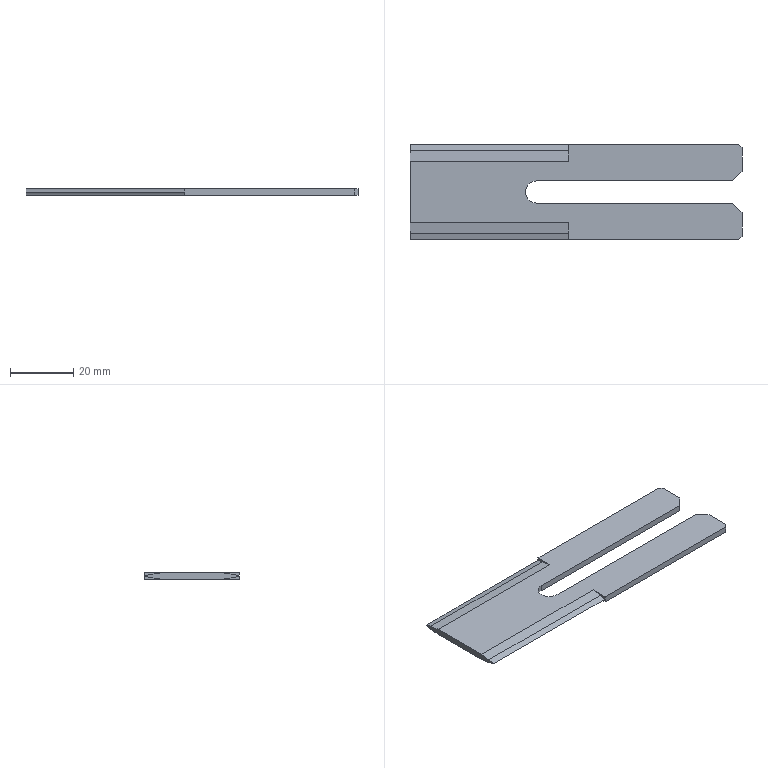Part | SolidWorks | features Chamfer 2, ICE 2, Extrusion 1 | 1 solid | 27 faces | box 105 x 30 x 2 mm | volume 4885 mm3 | plane 25 | cylinder 2 | commonest cylinder face diameters 7 x2
STEP:
#1=CARTESIAN_POINT('',(-16.,0.,2.));
#2=VERTEX_POINT('',#1);
#3=CARTESIAN_POINT('',(-12.5,3.5,2.));
#4=VERTEX_POINT('',#3);
#5=CARTESIAN_POINT('',(-12.5,0.,2.));
#6=DIRECTION('',(0.,0.,-1.));
#7=DIRECTION('',(1.,0.,0.));
#8=AXIS2_PLACEMENT_3D('',#5,#6,#7);
#9=CIRCLE('',#8,3.5);
#10=EDGE_CURVE('',#2,#4,#9,.T.);
#11=ORIENTED_EDGE('',*,*,#10,.F.);
#12=CARTESIAN_POINT('',(-16.,0.,0.));
#13=VERTEX_POINT('',#12);
#14=CARTESIAN_POINT('',(-16.,0.,141.025));
#15=DIRECTION('',(0.,0.,-1.));
#16=VECTOR('',#15,1000.);
#17=LINE('',#14,#16);
#18=EDGE_CURVE('',#2,#13,#17,.T.);
#19=ORIENTED_EDGE('',*,*,#18,.T.);
#20=CARTESIAN_POINT('',(-12.5,3.5,0.));
#21=VERTEX_POINT('',#20);
#22=CARTESIAN_POINT('',(-12.5,0.,0.));
#23=DIRECTION('',(0.,0.,-1.));
#24=DIRECTION('',(1.,0.,0.));
#25=AXIS2_PLACEMENT_3D('',#22,#23,#24);
#26=CIRCLE('',#25,3.5);
#27=EDGE_CURVE('',#13,#21,#26,.T.);
#28=ORIENTED_EDGE('',*,*,#27,.T.);
#29=CARTESIAN_POINT('',(-12.5,3.5,141.025));
#30=DIRECTION('',(0.,0.,-1.));
#31=VECTOR('',#30,1000.);
#32=LINE('',#29,#31);
#33=EDGE_CURVE('',#4,#21,#32,.T.);
#34=ORIENTED_EDGE('',*,*,#33,.F.);
#35=EDGE_LOOP('',(#11,#19,#28,#34));
#36=FACE_OUTER_BOUND('',#35,.T.);
#37=CARTESIAN_POINT('',(-12.5,0.,141.025));
#38=DIRECTION('',(0.,0.,-1.));
#39=DIRECTION('',(-1.,0.,0.));
#40=AXIS2_PLACEMENT_3D('',#37,#38,#39);
#41=CYLINDRICAL_SURFACE('',#40,3.5);
#42=ADVANCED_FACE('',(#36),#41,.F.);
#43=CARTESIAN_POINT('',(49.5,3.5,2.));
#44=VERTEX_POINT('',#43);
#45=CARTESIAN_POINT('',(0.,3.5,2.));
#46=DIRECTION('',(1.,0.,0.));
#47=VECTOR('',#46,1000.);
#48=LINE('',#45,#47);
#49=EDGE_CURVE('',#4,#44,#48,.T.);
#50=ORIENTED_EDGE('',*,*,#49,.T.);
#51=CARTESIAN_POINT('',(52.5,6.5,2.));
#52=VERTEX_POINT('',#51);
#53=CARTESIAN_POINT('',(23.,-23.,2.));
#54=DIRECTION('',(0.7071,0.7071,0.));
#55=VECTOR('',#54,1000.);
#56=LINE('',#53,#55);
#57=EDGE_CURVE('',#44,#52,#56,.T.);
#58=ORIENTED_EDGE('',*,*,#57,.T.);
#59=CARTESIAN_POINT('',(52.5,14.,2.));
#60=VERTEX_POINT('',#59);
#61=CARTESIAN_POINT('',(52.5,15.,2.));
#62=DIRECTION('',(0.,1.,0.));
#63=VECTOR('',#62,1000.);
#64=LINE('',#61,#63);
#65=EDGE_CURVE('',#52,#60,#64,.T.);
#66=ORIENTED_EDGE('',*,*,#65,.T.);
#67=CARTESIAN_POINT('',(51.5,15.,2.));
#68=VERTEX_POINT('',#67);
#69=CARTESIAN_POINT('',(33.25,33.25,2.));
#70=DIRECTION('',(-0.7071,0.7071,0.));
#71=VECTOR('',#70,1000.);
#72=LINE('',#69,#71);
#73=EDGE_CURVE('',#60,#68,#72,.T.);
#74=ORIENTED_EDGE('',*,*,#73,.T.);
#75=CARTESIAN_POINT('',(-2.5,15.,2.));
#76=VERTEX_POINT('',#75);
#77=CARTESIAN_POINT('',(-52.5,15.,2.));
#78=DIRECTION('',(-1.,0.,0.));
#79=VECTOR('',#78,1000.);
#80=LINE('',#77,#79);
#81=EDGE_CURVE('',#68,#76,#80,.T.);
#82=ORIENTED_EDGE('',*,*,#81,.T.);
#83=CARTESIAN_POINT('',(-2.5,9.698,2.));
#84=VERTEX_POINT('',#83);
#85=CARTESIAN_POINT('',(-2.5,0.,2.));
#86=DIRECTION('',(0.,-1.,0.));
#87=VECTOR('',#86,1000.);
#88=LINE('',#85,#87);
#89=EDGE_CURVE('',#76,#84,#88,.T.);
#90=ORIENTED_EDGE('',*,*,#89,.T.);
#91=CARTESIAN_POINT('',(-52.5,9.698,2.));
#92=VERTEX_POINT('',#91);
#93=CARTESIAN_POINT('',(-2.5,9.698,2.));
#94=DIRECTION('',(-1.,0.,0.));
#95=VECTOR('',#94,1000.);
#96=LINE('',#93,#95);
#97=EDGE_CURVE('',#84,#92,#96,.T.);
#98=ORIENTED_EDGE('',*,*,#97,.T.);
#99=CARTESIAN_POINT('',(-52.5,-9.698,2.));
#100=VERTEX_POINT('',#99);
#101=CARTESIAN_POINT('',(-52.5,15.,2.));
#102=DIRECTION('',(0.,-1.,0.));
#103=VECTOR('',#102,1000.);
#104=LINE('',#101,#103);
#105=EDGE_CURVE('',#92,#100,#104,.T.);
#106=ORIENTED_EDGE('',*,*,#105,.T.);
#107=CARTESIAN_POINT('',(-2.5,-9.698,2.));
#108=VERTEX_POINT('',#107);
#109=CARTESIAN_POINT('',(-2.5,-9.698,2.));
#110=DIRECTION('',(-1.,0.,0.));
#111=VECTOR('',#110,1000.);
#112=LINE('',#109,#111);
#113=EDGE_CURVE('',#108,#100,#112,.T.);
#114=ORIENTED_EDGE('',*,*,#113,.F.);
#115=CARTESIAN_POINT('',(-2.5,-15.,2.));
#116=VERTEX_POINT('',#115);
#117=CARTESIAN_POINT('',(-2.5,0.,2.));
#118=DIRECTION('',(0.,-1.,0.));
#119=VECTOR('',#118,1000.);
#120=LINE('',#117,#119);
#121=EDGE_CURVE('',#108,#116,#120,.T.);
#122=ORIENTED_EDGE('',*,*,#121,.T.);
#123=CARTESIAN_POINT('',(51.5,-15.,2.));
#124=VERTEX_POINT('',#123);
#125=CARTESIAN_POINT('',(-52.5,-15.,2.));
#126=DIRECTION('',(1.,0.,0.));
#127=VECTOR('',#126,1000.);
#128=LINE('',#125,#127);
#129=EDGE_CURVE('',#116,#124,#128,.T.);
#130=ORIENTED_EDGE('',*,*,#129,.T.);
#131=CARTESIAN_POINT('',(52.5,-14.,2.));
#132=VERTEX_POINT('',#131);
#133=CARTESIAN_POINT('',(33.25,-33.25,2.));
#134=DIRECTION('',(0.7071,0.7071,0.));
#135=VECTOR('',#134,1000.);
#136=LINE('',#133,#135);
#137=EDGE_CURVE('',#124,#132,#136,.T.);
#138=ORIENTED_EDGE('',*,*,#137,.T.);
#139=CARTESIAN_POINT('',(52.5,-6.5,2.));
#140=VERTEX_POINT('',#139);
#141=CARTESIAN_POINT('',(52.5,15.,2.));
#142=DIRECTION('',(0.,1.,0.));
#143=VECTOR('',#142,1000.);
#144=LINE('',#141,#143);
#145=EDGE_CURVE('',#132,#140,#144,.T.);
#146=ORIENTED_EDGE('',*,*,#145,.T.);
#147=CARTESIAN_POINT('',(49.5,-3.5,2.));
#148=VERTEX_POINT('',#147);
#149=CARTESIAN_POINT('',(23.,23.,2.));
#150=DIRECTION('',(-0.7071,0.7071,0.));
#151=VECTOR('',#150,1000.);
#152=LINE('',#149,#151);
#153=EDGE_CURVE('',#140,#148,#152,.T.);
#154=ORIENTED_EDGE('',*,*,#153,.T.);
#155=CARTESIAN_POINT('',(-12.5,-3.5,2.));
#156=VERTEX_POINT('',#155);
#157=CARTESIAN_POINT('',(0.,-3.5,2.));
#158=DIRECTION('',(-1.,0.,0.));
#159=VECTOR('',#158,1000.);
#160=LINE('',#157,#159);
#161=EDGE_CURVE('',#148,#156,#160,.T.);
#162=ORIENTED_EDGE('',*,*,#161,.T.);
#163=CARTESIAN_POINT('',(-12.5,0.,2.));
#164=DIRECTION('',(0.,0.,-1.));
#165=DIRECTION('',(1.,0.,0.));
#166=AXIS2_PLACEMENT_3D('',#163,#164,#165);
#167=CIRCLE('',#166,3.5);
#168=EDGE_CURVE('',#156,#2,#167,.T.);
#169=ORIENTED_EDGE('',*,*,#168,.T.);
#170=ORIENTED_EDGE('',*,*,#10,.T.);
#171=EDGE_LOOP('',(#50,#58,#66,#74,#82,#90,#98,#106,#114,#122,#130,#138,#146,#154,#162,#169,#170));
#172=FACE_OUTER_BOUND('',#171,.T.);
#173=CARTESIAN_POINT('',(0.,0.,2.));
#174=DIRECTION('',(0.,0.,1.));
#175=DIRECTION('',(1.,0.,0.));
#176=AXIS2_PLACEMENT_3D('',#173,#174,#175);
#177=PLANE('',#176);
#178=ADVANCED_FACE('',(#172),#177,.T.);
#179=CARTESIAN_POINT('',(52.5,6.5,0.));
#180=VERTEX_POINT('',#179);
#181=CARTESIAN_POINT('',(52.5,14.,0.));
#182=VERTEX_POINT('',#181);
#183=CARTESIAN_POINT('',(52.5,15.,0.));
#184=DIRECTION('',(0.,1.,0.));
#185=VECTOR('',#184,1000.);
#186=LINE('',#183,#185);
#187=EDGE_CURVE('',#180,#182,#186,.T.);
#188=ORIENTED_EDGE('',*,*,#187,.F.);
#189=CARTESIAN_POINT('',(49.5,3.5,0.));
#190=VERTEX_POINT('',#189);
#191=CARTESIAN_POINT('',(52.5,6.5,0.));
#192=DIRECTION('',(-0.7071,-0.7071,0.));
#193=VECTOR('',#192,1000.);
#194=LINE('',#191,#193);
#195=EDGE_CURVE('',#180,#190,#194,.T.);
#196=ORIENTED_EDGE('',*,*,#195,.T.);
#197=CARTESIAN_POINT('',(0.,3.5,0.));
#198=DIRECTION('',(1.,0.,0.));
#199=VECTOR('',#198,1000.);
#200=LINE('',#197,#199);
#201=EDGE_CURVE('',#21,#190,#200,.T.);
#202=ORIENTED_EDGE('',*,*,#201,.F.);
#203=ORIENTED_EDGE('',*,*,#27,.F.);
#204=CARTESIAN_POINT('',(-12.5,-3.5,0.));
#205=VERTEX_POINT('',#204);
#206=CARTESIAN_POINT('',(-12.5,0.,0.));
#207=DIRECTION('',(0.,0.,-1.));
#208=DIRECTION('',(1.,0.,0.));
#209=AXIS2_PLACEMENT_3D('',#206,#207,#208);
#210=CIRCLE('',#209,3.5);
#211=EDGE_CURVE('',#205,#13,#210,.T.);
#212=ORIENTED_EDGE('',*,*,#211,.F.);
#213=CARTESIAN_POINT('',(49.5,-3.5,0.));
#214=VERTEX_POINT('',#213);
#215=CARTESIAN_POINT('',(0.,-3.5,0.));
#216=DIRECTION('',(-1.,0.,0.));
#217=VECTOR('',#216,1000.);
#218=LINE('',#215,#217);
#219=EDGE_CURVE('',#214,#205,#218,.T.);
#220=ORIENTED_EDGE('',*,*,#219,.F.);
#221=CARTESIAN_POINT('',(52.5,-6.5,0.));
#222=VERTEX_POINT('',#221);
#223=CARTESIAN_POINT('',(49.5,-3.5,0.));
#224=DIRECTION('',(0.7071,-0.7071,0.));
#225=VECTOR('',#224,1000.);
#226=LINE('',#223,#225);
#227=EDGE_CURVE('',#214,#222,#226,.T.);
#228=ORIENTED_EDGE('',*,*,#227,.T.);
#229=CARTESIAN_POINT('',(52.5,-14.,0.));
#230=VERTEX_POINT('',#229);
#231=CARTESIAN_POINT('',(52.5,15.,0.));
#232=DIRECTION('',(0.,1.,0.));
#233=VECTOR('',#232,1000.);
#234=LINE('',#231,#233);
#235=EDGE_CURVE('',#230,#222,#234,.T.);
#236=ORIENTED_EDGE('',*,*,#235,.F.);
#237=CARTESIAN_POINT('',(51.5,-15.,0.));
#238=VERTEX_POINT('',#237);
#239=CARTESIAN_POINT('',(52.5,-14.,0.));
#240=DIRECTION('',(-0.7071,-0.7071,0.));
#241=VECTOR('',#240,1000.);
#242=LINE('',#239,#241);
#243=EDGE_CURVE('',#230,#238,#242,.T.);
#244=ORIENTED_EDGE('',*,*,#243,.T.);
#245=CARTESIAN_POINT('',(-2.5,-15.,0.));
#246=VERTEX_POINT('',#245);
#247=CARTESIAN_POINT('',(-52.5,-15.,0.));
#248=DIRECTION('',(1.,0.,0.));
#249=VECTOR('',#248,1000.);
#250=LINE('',#247,#249);
#251=EDGE_CURVE('',#246,#238,#250,.T.);
#252=ORIENTED_EDGE('',*,*,#251,.F.);
#253=CARTESIAN_POINT('',(-2.5,-9.698,0.));
#254=VERTEX_POINT('',#253);
#255=CARTESIAN_POINT('',(-2.5,0.,0.));
#256=DIRECTION('',(0.,-1.,0.));
#257=VECTOR('',#256,1000.);
#258=LINE('',#255,#257);
#259=EDGE_CURVE('',#254,#246,#258,.T.);
#260=ORIENTED_EDGE('',*,*,#259,.F.);
#261=CARTESIAN_POINT('',(-52.5,-9.698,0.));
#262=VERTEX_POINT('',#261);
#263=CARTESIAN_POINT('',(-2.5,-9.698,0.));
#264=DIRECTION('',(-1.,0.,0.));
#265=VECTOR('',#264,1000.);
#266=LINE('',#263,#265);
#267=EDGE_CURVE('',#254,#262,#266,.T.);
#268=ORIENTED_EDGE('',*,*,#267,.T.);
#269=CARTESIAN_POINT('',(-52.5,9.698,0.));
#270=VERTEX_POINT('',#269);
#271=CARTESIAN_POINT('',(-52.5,15.,0.));
#272=DIRECTION('',(0.,-1.,0.));
#273=VECTOR('',#272,1000.);
#274=LINE('',#271,#273);
#275=EDGE_CURVE('',#270,#262,#274,.T.);
#276=ORIENTED_EDGE('',*,*,#275,.F.);
#277=CARTESIAN_POINT('',(-2.5,9.698,0.));
#278=VERTEX_POINT('',#277);
#279=CARTESIAN_POINT('',(-2.5,9.698,0.));
#280=DIRECTION('',(-1.,0.,0.));
#281=VECTOR('',#280,1000.);
#282=LINE('',#279,#281);
#283=EDGE_CURVE('',#278,#270,#282,.T.);
#284=ORIENTED_EDGE('',*,*,#283,.F.);
#285=CARTESIAN_POINT('',(-2.5,15.,0.));
#286=VERTEX_POINT('',#285);
#287=CARTESIAN_POINT('',(-2.5,0.,0.));
#288=DIRECTION('',(0.,-1.,0.));
#289=VECTOR('',#288,1000.);
#290=LINE('',#287,#289);
#291=EDGE_CURVE('',#286,#278,#290,.T.);
#292=ORIENTED_EDGE('',*,*,#291,.F.);
#293=CARTESIAN_POINT('',(51.5,15.,0.));
#294=VERTEX_POINT('',#293);
#295=CARTESIAN_POINT('',(-52.5,15.,0.));
#296=DIRECTION('',(-1.,0.,0.));
#297=VECTOR('',#296,1000.);
#298=LINE('',#295,#297);
#299=EDGE_CURVE('',#294,#286,#298,.T.);
#300=ORIENTED_EDGE('',*,*,#299,.F.);
#301=CARTESIAN_POINT('',(51.5,15.,0.));
#302=DIRECTION('',(0.7071,-0.7071,0.));
#303=VECTOR('',#302,1000.);
#304=LINE('',#301,#303);
#305=EDGE_CURVE('',#294,#182,#304,.T.);
#306=ORIENTED_EDGE('',*,*,#305,.T.);
#307=EDGE_LOOP('',(#188,#196,#202,#203,#212,#220,#228,#236,#244,#252,#260,#268,#276,#284,#292,#300,#306));
#308=FACE_OUTER_BOUND('',#307,.T.);
#309=CARTESIAN_POINT('',(0.,0.,0.));
#310=DIRECTION('',(0.,0.,1.));
#311=DIRECTION('',(1.,0.,0.));
#312=AXIS2_PLACEMENT_3D('',#309,#310,#311);
#313=PLANE('',#312);
#314=ADVANCED_FACE('',(#308),#313,.F.);
#315=ORIENTED_EDGE('',*,*,#81,.F.);
#316=CARTESIAN_POINT('',(51.5,15.,2.));
#317=DIRECTION('',(0.,0.,-1.));
#318=VECTOR('',#317,1000.);
#319=LINE('',#316,#318);
#320=EDGE_CURVE('',#68,#294,#319,.T.);
#321=ORIENTED_EDGE('',*,*,#320,.T.);
#322=ORIENTED_EDGE('',*,*,#299,.T.);
#323=CARTESIAN_POINT('',(-2.5,15.,1.));
#324=VERTEX_POINT('',#323);
#325=CARTESIAN_POINT('',(-2.5,15.,2.));
#326=DIRECTION('',(0.,0.,-1.));
#327=VECTOR('',#326,1000.);
#328=LINE('',#325,#327);
#329=EDGE_CURVE('',#324,#286,#328,.T.);
#330=ORIENTED_EDGE('',*,*,#329,.F.);
#331=CARTESIAN_POINT('',(-2.5,15.,2.));
#332=DIRECTION('',(0.,0.,-1.));
#333=VECTOR('',#332,1000.);
#334=LINE('',#331,#333);
#335=EDGE_CURVE('',#76,#324,#334,.T.);
#336=ORIENTED_EDGE('',*,*,#335,.F.);
#337=EDGE_LOOP('',(#315,#321,#322,#330,#336));
#338=FACE_OUTER_BOUND('',#337,.T.);
#339=CARTESIAN_POINT('',(-52.5,15.,2.));
#340=DIRECTION('',(0.,-1.,0.));
#341=DIRECTION('',(0.,0.,-1.));
#342=AXIS2_PLACEMENT_3D('',#339,#340,#341);
#343=PLANE('',#342);
#344=ADVANCED_FACE('',(#338),#343,.F.);
#345=CARTESIAN_POINT('',(-52.5,-13.,1.536));
#346=VERTEX_POINT('',#345);
#347=CARTESIAN_POINT('',(-52.5,-13.,1.536));
#348=DIRECTION('',(0.,0.9903,0.1392));
#349=VECTOR('',#348,1000.);
#350=LINE('',#347,#349);
#351=EDGE_CURVE('',#346,#100,#350,.T.);
#352=ORIENTED_EDGE('',*,*,#351,.T.);
#353=ORIENTED_EDGE('',*,*,#105,.F.);
#354=CARTESIAN_POINT('',(-52.5,13.,1.536));
#355=VERTEX_POINT('',#354);
#356=CARTESIAN_POINT('',(-52.5,13.,1.536));
#357=DIRECTION('',(0.,0.9903,-0.1392));
#358=VECTOR('',#357,1000.);
#359=LINE('',#356,#358);
#360=EDGE_CURVE('',#92,#355,#359,.T.);
#361=ORIENTED_EDGE('',*,*,#360,.T.);
#362=CARTESIAN_POINT('',(-52.5,15.,1.));
#363=VERTEX_POINT('',#362);
#364=CARTESIAN_POINT('',(-52.5,15.,1.));
#365=DIRECTION('',(0.,0.9659,-0.2588));
#366=VECTOR('',#365,1000.);
#367=LINE('',#364,#366);
#368=EDGE_CURVE('',#355,#363,#367,.T.);
#369=ORIENTED_EDGE('',*,*,#368,.T.);
#370=CARTESIAN_POINT('',(-52.5,13.,0.4641));
#371=VERTEX_POINT('',#370);
#372=CARTESIAN_POINT('',(-52.5,15.,1.));
#373=DIRECTION('',(0.,-0.9659,-0.2588));
#374=VECTOR('',#373,1000.);
#375=LINE('',#372,#374);
#376=EDGE_CURVE('',#363,#371,#375,.T.);
#377=ORIENTED_EDGE('',*,*,#376,.T.);
#378=CARTESIAN_POINT('',(-52.5,13.,0.4641));
#379=DIRECTION('',(0.,-0.9903,-0.1392));
#380=VECTOR('',#379,1000.);
#381=LINE('',#378,#380);
#382=EDGE_CURVE('',#371,#270,#381,.T.);
#383=ORIENTED_EDGE('',*,*,#382,.T.);
#384=ORIENTED_EDGE('',*,*,#275,.T.);
#385=CARTESIAN_POINT('',(-52.5,-13.,0.4641));
#386=VERTEX_POINT('',#385);
#387=CARTESIAN_POINT('',(-52.5,-13.,0.4641));
#388=DIRECTION('',(0.,-0.9903,0.1392));
#389=VECTOR('',#388,1000.);
#390=LINE('',#387,#389);
#391=EDGE_CURVE('',#262,#386,#390,.T.);
#392=ORIENTED_EDGE('',*,*,#391,.T.);
#393=CARTESIAN_POINT('',(-52.5,-15.,1.));
#394=VERTEX_POINT('',#393);
#395=CARTESIAN_POINT('',(-52.5,-15.,1.));
#396=DIRECTION('',(0.,-0.9659,0.2588));
#397=VECTOR('',#396,1000.);
#398=LINE('',#395,#397);
#399=EDGE_CURVE('',#386,#394,#398,.T.);
#400=ORIENTED_EDGE('',*,*,#399,.T.);
#401=CARTESIAN_POINT('',(-52.5,-15.,1.));
#402=DIRECTION('',(0.,0.9659,0.2588));
#403=VECTOR('',#402,1000.);
#404=LINE('',#401,#403);
#405=EDGE_CURVE('',#394,#346,#404,.T.);
#406=ORIENTED_EDGE('',*,*,#405,.T.);
#407=EDGE_LOOP('',(#352,#353,#361,#369,#377,#383,#384,#392,#400,#406));
#408=FACE_OUTER_BOUND('',#407,.T.);
#409=CARTESIAN_POINT('',(-52.5,15.,2.));
#410=DIRECTION('',(1.,0.,0.));
#411=DIRECTION('',(0.,1.,0.));
#412=AXIS2_PLACEMENT_3D('',#409,#410,#411);
#413=PLANE('',#412);
#414=ADVANCED_FACE('',(#408),#413,.F.);
#415=ORIENTED_EDGE('',*,*,#251,.T.);
#416=CARTESIAN_POINT('',(51.5,-15.,2.));
#417=DIRECTION('',(0.,0.,1.));
#418=VECTOR('',#417,1000.);
#419=LINE('',#416,#418);
#420=EDGE_CURVE('',#238,#124,#419,.T.);
#421=ORIENTED_EDGE('',*,*,#420,.T.);
#422=ORIENTED_EDGE('',*,*,#129,.F.);
#423=CARTESIAN_POINT('',(-2.5,-15.,1.));
#424=VERTEX_POINT('',#423);
#425=CARTESIAN_POINT('',(-2.5,-15.,2.));
#426=DIRECTION('',(0.,0.,1.));
#427=VECTOR('',#426,1000.);
#428=LINE('',#425,#427);
#429=EDGE_CURVE('',#424,#116,#428,.T.);
#430=ORIENTED_EDGE('',*,*,#429,.F.);
#431=CARTESIAN_POINT('',(-2.5,-15.,2.));
#432=DIRECTION('',(0.,0.,1.));
#433=VECTOR('',#432,1000.);
#434=LINE('',#431,#433);
#435=EDGE_CURVE('',#246,#424,#434,.T.);
#436=ORIENTED_EDGE('',*,*,#435,.F.);
#437=EDGE_LOOP('',(#415,#421,#422,#430,#436));
#438=FACE_OUTER_BOUND('',#437,.T.);
#439=CARTESIAN_POINT('',(-52.5,-15.,2.));
#440=DIRECTION('',(0.,1.,0.));
#441=DIRECTION('',(0.,0.,1.));
#442=AXIS2_PLACEMENT_3D('',#439,#440,#441);
#443=PLANE('',#442);
#444=ADVANCED_FACE('',(#438),#443,.F.);
#445=ORIENTED_EDGE('',*,*,#65,.F.);
#446=CARTESIAN_POINT('',(52.5,6.5,0.));
#447=DIRECTION('',(0.,0.,-1.));
#448=VECTOR('',#447,1000.);
#449=LINE('',#446,#448);
#450=EDGE_CURVE('',#52,#180,#449,.T.);
#451=ORIENTED_EDGE('',*,*,#450,.T.);
#452=ORIENTED_EDGE('',*,*,#187,.T.);
#453=CARTESIAN_POINT('',(52.5,14.,2.));
#454=DIRECTION('',(0.,0.,1.));
#455=VECTOR('',#454,1000.);
#456=LINE('',#453,#455);
#457=EDGE_CURVE('',#182,#60,#456,.T.);
#458=ORIENTED_EDGE('',*,*,#457,.T.);
#459=EDGE_LOOP('',(#445,#451,#452,#458));
#460=FACE_OUTER_BOUND('',#459,.T.);
#461=CARTESIAN_POINT('',(52.5,15.,2.));
#462=DIRECTION('',(-1.,0.,0.));
#463=DIRECTION('',(0.,0.,1.));
#464=AXIS2_PLACEMENT_3D('',#461,#462,#463);
#465=PLANE('',#464);
#466=ADVANCED_FACE('',(#460),#465,.F.);
#467=ORIENTED_EDGE('',*,*,#235,.T.);
#468=CARTESIAN_POINT('',(52.5,-6.5,2.));
#469=DIRECTION('',(0.,0.,1.));
#470=VECTOR('',#469,1000.);
#471=LINE('',#468,#470);
#472=EDGE_CURVE('',#222,#140,#471,.T.);
#473=ORIENTED_EDGE('',*,*,#472,.T.);
#474=ORIENTED_EDGE('',*,*,#145,.F.);
#475=CARTESIAN_POINT('',(52.5,-14.,2.));
#476=DIRECTION('',(0.,0.,-1.));
#477=VECTOR('',#476,1000.);
#478=LINE('',#475,#477);
#479=EDGE_CURVE('',#132,#230,#478,.T.);
#480=ORIENTED_EDGE('',*,*,#479,.T.);
#481=EDGE_LOOP('',(#467,#473,#474,#480));
#482=FACE_OUTER_BOUND('',#481,.T.);
#483=CARTESIAN_POINT('',(52.5,15.,2.));
#484=DIRECTION('',(-1.,0.,0.));
#485=DIRECTION('',(0.,0.,1.));
#486=AXIS2_PLACEMENT_3D('',#483,#484,#485);
#487=PLANE('',#486);
#488=ADVANCED_FACE('',(#482),#487,.F.);
#489=ORIENTED_EDGE('',*,*,#201,.T.);
#490=CARTESIAN_POINT('',(49.5,3.5,2.));
#491=DIRECTION('',(0.,0.,1.));
#492=VECTOR('',#491,1000.);
#493=LINE('',#490,#492);
#494=EDGE_CURVE('',#190,#44,#493,.T.);
#495=ORIENTED_EDGE('',*,*,#494,.T.);
#496=ORIENTED_EDGE('',*,*,#49,.F.);
#497=ORIENTED_EDGE('',*,*,#33,.T.);
#498=EDGE_LOOP('',(#489,#495,#496,#497));
#499=FACE_OUTER_BOUND('',#498,.T.);
#500=CARTESIAN_POINT('',(-12.5,3.5,141.025));
#501=DIRECTION('',(0.,-1.,0.));
#502=DIRECTION('',(1.,0.,0.));
#503=AXIS2_PLACEMENT_3D('',#500,#501,#502);
#504=PLANE('',#503);
#505=ADVANCED_FACE('',(#499),#504,.T.);
#506=ORIENTED_EDGE('',*,*,#18,.F.);
#507=ORIENTED_EDGE('',*,*,#168,.F.);
#508=CARTESIAN_POINT('',(-12.5,-3.5,141.025));
#509=DIRECTION('',(0.,0.,-1.));
#510=VECTOR('',#509,1000.);
#511=LINE('',#508,#510);
#512=EDGE_CURVE('',#156,#205,#511,.T.);
#513=ORIENTED_EDGE('',*,*,#512,.T.);
#514=ORIENTED_EDGE('',*,*,#211,.T.);
#515=EDGE_LOOP('',(#506,#507,#513,#514));
#516=FACE_OUTER_BOUND('',#515,.T.);
#517=CARTESIAN_POINT('',(-12.5,0.,141.025));
#518=DIRECTION('',(0.,0.,-1.));
#519=DIRECTION('',(-1.,0.,0.));
#520=AXIS2_PLACEMENT_3D('',#517,#518,#519);
#521=CYLINDRICAL_SURFACE('',#520,3.5);
#522=ADVANCED_FACE('',(#516),#521,.F.);
#523=ORIENTED_EDGE('',*,*,#161,.F.);
#524=CARTESIAN_POINT('',(49.5,-3.5,0.));
#525=DIRECTION('',(0.,0.,-1.));
#526=VECTOR('',#525,1000.);
#527=LINE('',#524,#526);
#528=EDGE_CURVE('',#148,#214,#527,.T.);
#529=ORIENTED_EDGE('',*,*,#528,.T.);
#530=ORIENTED_EDGE('',*,*,#219,.T.);
#531=ORIENTED_EDGE('',*,*,#512,.F.);
#532=EDGE_LOOP('',(#523,#529,#530,#531));
#533=FACE_OUTER_BOUND('',#532,.T.);
#534=CARTESIAN_POINT('',(-12.5,-3.5,141.025));
#535=DIRECTION('',(0.,1.,0.));
#536=DIRECTION('',(-1.,0.,0.));
#537=AXIS2_PLACEMENT_3D('',#534,#535,#536);
#538=PLANE('',#537);
#539=ADVANCED_FACE('',(#533),#538,.T.);
#540=ORIENTED_EDGE('',*,*,#259,.T.);
#541=ORIENTED_EDGE('',*,*,#435,.T.);
#542=CARTESIAN_POINT('',(-2.5,-13.,0.4641));
#543=VERTEX_POINT('',#542);
#544=CARTESIAN_POINT('',(-2.5,-15.,1.));
#545=DIRECTION('',(0.,-0.9659,0.2588));
#546=VECTOR('',#545,1000.);
#547=LINE('',#544,#546);
#548=EDGE_CURVE('',#543,#424,#547,.T.);
#549=ORIENTED_EDGE('',*,*,#548,.F.);
#550=CARTESIAN_POINT('',(-2.5,-13.,0.4641));
#551=DIRECTION('',(0.,-0.9903,0.1392));
#552=VECTOR('',#551,1000.);
#553=LINE('',#550,#552);
#554=EDGE_CURVE('',#254,#543,#553,.T.);
#555=ORIENTED_EDGE('',*,*,#554,.F.);
#556=EDGE_LOOP('',(#540,#541,#549,#555));
#557=FACE_OUTER_BOUND('',#556,.T.);
#558=CARTESIAN_POINT('',(-2.5,-0.3973,1.073));
#559=DIRECTION('',(-1.,0.,0.));
#560=DIRECTION('',(0.,-1.,0.));
#561=AXIS2_PLACEMENT_3D('',#558,#559,#560);
#562=PLANE('',#561);
#563=ADVANCED_FACE('',(#557),#562,.T.);
#564=ORIENTED_EDGE('',*,*,#391,.F.);
#565=ORIENTED_EDGE('',*,*,#267,.F.);
#566=ORIENTED_EDGE('',*,*,#554,.T.);
#567=CARTESIAN_POINT('',(-2.5,-13.,0.4641));
#568=DIRECTION('',(-1.,0.,0.));
#569=VECTOR('',#568,1000.);
#570=LINE('',#567,#569);
#571=EDGE_CURVE('',#543,#386,#570,.T.);
#572=ORIENTED_EDGE('',*,*,#571,.T.);
#573=EDGE_LOOP('',(#564,#565,#566,#572));
#574=FACE_OUTER_BOUND('',#573,.T.);
#575=CARTESIAN_POINT('',(-2.5,-13.,0.4641));
#576=DIRECTION('',(0.,-0.1392,-0.9903));
#577=DIRECTION('',(0.,0.9903,-0.1392));
#578=AXIS2_PLACEMENT_3D('',#575,#576,#577);
#579=PLANE('',#578);
#580=ADVANCED_FACE('',(#574),#579,.T.);
#581=ORIENTED_EDGE('',*,*,#399,.F.);
#582=ORIENTED_EDGE('',*,*,#571,.F.);
#583=ORIENTED_EDGE('',*,*,#548,.T.);
#584=CARTESIAN_POINT('',(-2.5,-15.,1.));
#585=DIRECTION('',(-1.,0.,0.));
#586=VECTOR('',#585,1000.);
#587=LINE('',#584,#586);
#588=EDGE_CURVE('',#424,#394,#587,.T.);
#589=ORIENTED_EDGE('',*,*,#588,.T.);
#590=EDGE_LOOP('',(#581,#582,#583,#589));
#591=FACE_OUTER_BOUND('',#590,.T.);
#592=CARTESIAN_POINT('',(-2.5,-15.,1.));
#593=DIRECTION('',(0.,-0.2588,-0.9659));
#594=DIRECTION('',(0.,0.9659,-0.2588));
#595=AXIS2_PLACEMENT_3D('',#592,#593,#594);
#596=PLANE('',#595);
#597=ADVANCED_FACE('',(#591),#596,.T.);
#598=CARTESIAN_POINT('',(-2.5,-13.,1.536));
#599=VERTEX_POINT('',#598);
#600=CARTESIAN_POINT('',(-2.5,-13.,1.536));
#601=DIRECTION('',(0.,0.9903,0.1392));
#602=VECTOR('',#601,1000.);
#603=LINE('',#600,#602);
#604=EDGE_CURVE('',#599,#108,#603,.T.);
#605=ORIENTED_EDGE('',*,*,#604,.F.);
#606=CARTESIAN_POINT('',(-2.5,-15.,1.));
#607=DIRECTION('',(0.,0.9659,0.2588));
#608=VECTOR('',#607,1000.);
#609=LINE('',#606,#608);
#610=EDGE_CURVE('',#424,#599,#609,.T.);
#611=ORIENTED_EDGE('',*,*,#610,.F.);
#612=ORIENTED_EDGE('',*,*,#429,.T.);
#613=ORIENTED_EDGE('',*,*,#121,.F.);
#614=EDGE_LOOP('',(#605,#611,#612,#613));
#615=FACE_OUTER_BOUND('',#614,.T.);
#616=CARTESIAN_POINT('',(-2.5,-0.3973,1.073));
#617=DIRECTION('',(-1.,0.,0.));
#618=DIRECTION('',(0.,-1.,0.));
#619=AXIS2_PLACEMENT_3D('',#616,#617,#618);
#620=PLANE('',#619);
#621=ADVANCED_FACE('',(#615),#620,.T.);
#622=ORIENTED_EDGE('',*,*,#405,.F.);
#623=ORIENTED_EDGE('',*,*,#588,.F.);
#624=ORIENTED_EDGE('',*,*,#610,.T.);
#625=CARTESIAN_POINT('',(-2.5,-13.,1.536));
#626=DIRECTION('',(-1.,0.,0.));
#627=VECTOR('',#626,1000.);
#628=LINE('',#625,#627);
#629=EDGE_CURVE('',#599,#346,#628,.T.);
#630=ORIENTED_EDGE('',*,*,#629,.T.);
#631=EDGE_LOOP('',(#622,#623,#624,#630));
#632=FACE_OUTER_BOUND('',#631,.T.);
#633=CARTESIAN_POINT('',(-2.5,-15.,1.));
#634=DIRECTION('',(0.,-0.2588,0.9659));
#635=DIRECTION('',(0.,-0.9659,-0.2588));
#636=AXIS2_PLACEMENT_3D('',#633,#634,#635);
#637=PLANE('',#636);
#638=ADVANCED_FACE('',(#632),#637,.T.);
#639=ORIENTED_EDGE('',*,*,#351,.F.);
#640=ORIENTED_EDGE('',*,*,#629,.F.);
#641=ORIENTED_EDGE('',*,*,#604,.T.);
#642=ORIENTED_EDGE('',*,*,#113,.T.);
#643=EDGE_LOOP('',(#639,#640,#641,#642));
#644=FACE_OUTER_BOUND('',#643,.T.);
#645=CARTESIAN_POINT('',(-2.5,-13.,1.536));
#646=DIRECTION('',(0.,-0.1392,0.9903));
#647=DIRECTION('',(0.,-0.9903,-0.1392));
#648=AXIS2_PLACEMENT_3D('',#645,#646,#647);
#649=PLANE('',#648);
#650=ADVANCED_FACE('',(#644),#649,.T.);
#651=ORIENTED_EDGE('',*,*,#291,.T.);
#652=CARTESIAN_POINT('',(-2.5,13.,0.4641));
#653=VERTEX_POINT('',#652);
#654=CARTESIAN_POINT('',(-2.5,13.,0.4641));
#655=DIRECTION('',(0.,-0.9903,-0.1392));
#656=VECTOR('',#655,1000.);
#657=LINE('',#654,#656);
#658=EDGE_CURVE('',#653,#278,#657,.T.);
#659=ORIENTED_EDGE('',*,*,#658,.F.);
#660=CARTESIAN_POINT('',(-2.5,15.,1.));
#661=DIRECTION('',(0.,-0.9659,-0.2588));
#662=VECTOR('',#661,1000.);
#663=LINE('',#660,#662);
#664=EDGE_CURVE('',#324,#653,#663,.T.);
#665=ORIENTED_EDGE('',*,*,#664,.F.);
#666=ORIENTED_EDGE('',*,*,#329,.T.);
#667=EDGE_LOOP('',(#651,#659,#665,#666));
#668=FACE_OUTER_BOUND('',#667,.T.);
#669=CARTESIAN_POINT('',(-2.5,-0.3973,1.073));
#670=DIRECTION('',(-1.,0.,0.));
#671=DIRECTION('',(0.,-1.,0.));
#672=AXIS2_PLACEMENT_3D('',#669,#670,#671);
#673=PLANE('',#672);
#674=ADVANCED_FACE('',(#668),#673,.T.);
#675=ORIENTED_EDGE('',*,*,#335,.T.);
#676=CARTESIAN_POINT('',(-2.5,13.,1.536));
#677=VERTEX_POINT('',#676);
#678=CARTESIAN_POINT('',(-2.5,15.,1.));
#679=DIRECTION('',(0.,0.9659,-0.2588));
#680=VECTOR('',#679,1000.);
#681=LINE('',#678,#680);
#682=EDGE_CURVE('',#677,#324,#681,.T.);
#683=ORIENTED_EDGE('',*,*,#682,.F.);
#684=CARTESIAN_POINT('',(-2.5,13.,1.536));
#685=DIRECTION('',(0.,0.9903,-0.1392));
#686=VECTOR('',#685,1000.);
#687=LINE('',#684,#686);
#688=EDGE_CURVE('',#84,#677,#687,.T.);
#689=ORIENTED_EDGE('',*,*,#688,.F.);
#690=ORIENTED_EDGE('',*,*,#89,.F.);
#691=EDGE_LOOP('',(#675,#683,#689,#690));
#692=FACE_OUTER_BOUND('',#691,.T.);
#693=CARTESIAN_POINT('',(-2.5,-0.3973,1.073));
#694=DIRECTION('',(-1.,0.,0.));
#695=DIRECTION('',(0.,-1.,0.));
#696=AXIS2_PLACEMENT_3D('',#693,#694,#695);
#697=PLANE('',#696);
#698=ADVANCED_FACE('',(#692),#697,.T.);
#699=ORIENTED_EDGE('',*,*,#368,.F.);
#700=CARTESIAN_POINT('',(-2.5,13.,1.536));
#701=DIRECTION('',(-1.,0.,0.));
#702=VECTOR('',#701,1000.);
#703=LINE('',#700,#702);
#704=EDGE_CURVE('',#677,#355,#703,.T.);
#705=ORIENTED_EDGE('',*,*,#704,.F.);
#706=ORIENTED_EDGE('',*,*,#682,.T.);
#707=CARTESIAN_POINT('',(-2.5,15.,1.));
#708=DIRECTION('',(-1.,0.,0.));
#709=VECTOR('',#708,1000.);
#710=LINE('',#707,#709);
#711=EDGE_CURVE('',#324,#363,#710,.T.);
#712=ORIENTED_EDGE('',*,*,#711,.T.);
#713=EDGE_LOOP('',(#699,#705,#706,#712));
#714=FACE_OUTER_BOUND('',#713,.T.);
#715=CARTESIAN_POINT('',(-2.5,15.,1.));
#716=DIRECTION('',(0.,0.2588,0.9659));
#717=DIRECTION('',(0.,-0.9659,0.2588));
#718=AXIS2_PLACEMENT_3D('',#715,#716,#717);
#719=PLANE('',#718);
#720=ADVANCED_FACE('',(#714),#719,.T.);
#721=ORIENTED_EDGE('',*,*,#360,.F.);
#722=ORIENTED_EDGE('',*,*,#97,.F.);
#723=ORIENTED_EDGE('',*,*,#688,.T.);
#724=ORIENTED_EDGE('',*,*,#704,.T.);
#725=EDGE_LOOP('',(#721,#722,#723,#724));
#726=FACE_OUTER_BOUND('',#725,.T.);
#727=CARTESIAN_POINT('',(-2.5,13.,1.536));
#728=DIRECTION('',(0.,0.1392,0.9903));
#729=DIRECTION('',(0.,-0.9903,0.1392));
#730=AXIS2_PLACEMENT_3D('',#727,#728,#729);
#731=PLANE('',#730);
#732=ADVANCED_FACE('',(#726),#731,.T.);
#733=ORIENTED_EDGE('',*,*,#382,.F.);
#734=CARTESIAN_POINT('',(-2.5,13.,0.4641));
#735=DIRECTION('',(-1.,0.,0.));
#736=VECTOR('',#735,1000.);
#737=LINE('',#734,#736);
#738=EDGE_CURVE('',#653,#371,#737,.T.);
#739=ORIENTED_EDGE('',*,*,#738,.F.);
#740=ORIENTED_EDGE('',*,*,#658,.T.);
#741=ORIENTED_EDGE('',*,*,#283,.T.);
#742=EDGE_LOOP('',(#733,#739,#740,#741));
#743=FACE_OUTER_BOUND('',#742,.T.);
#744=CARTESIAN_POINT('',(-2.5,13.,0.4641));
#745=DIRECTION('',(0.,0.1392,-0.9903));
#746=DIRECTION('',(0.,0.9903,0.1392));
#747=AXIS2_PLACEMENT_3D('',#744,#745,#746);
#748=PLANE('',#747);
#749=ADVANCED_FACE('',(#743),#748,.T.);
#750=ORIENTED_EDGE('',*,*,#376,.F.);
#751=ORIENTED_EDGE('',*,*,#711,.F.);
#752=ORIENTED_EDGE('',*,*,#664,.T.);
#753=ORIENTED_EDGE('',*,*,#738,.T.);
#754=EDGE_LOOP('',(#750,#751,#752,#753));
#755=FACE_OUTER_BOUND('',#754,.T.);
#756=CARTESIAN_POINT('',(-2.5,15.,1.));
#757=DIRECTION('',(0.,0.2588,-0.9659));
#758=DIRECTION('',(0.,0.9659,0.2588));
#759=AXIS2_PLACEMENT_3D('',#756,#757,#758);
#760=PLANE('',#759);
#761=ADVANCED_FACE('',(#755),#760,.T.);
#762=ORIENTED_EDGE('',*,*,#137,.F.);
#763=ORIENTED_EDGE('',*,*,#420,.F.);
#764=ORIENTED_EDGE('',*,*,#243,.F.);
#765=ORIENTED_EDGE('',*,*,#479,.F.);
#766=EDGE_LOOP('',(#762,#763,#764,#765));
#767=FACE_OUTER_BOUND('',#766,.T.);
#768=CARTESIAN_POINT('',(52.5,-14.,2.));
#769=DIRECTION('',(-0.7071,0.7071,0.));
#770=DIRECTION('',(0.,0.,-1.));
#771=AXIS2_PLACEMENT_3D('',#768,#769,#770);
#772=PLANE('',#771);
#773=ADVANCED_FACE('',(#767),#772,.F.);
#774=ORIENTED_EDGE('',*,*,#73,.F.);
#775=ORIENTED_EDGE('',*,*,#457,.F.);
#776=ORIENTED_EDGE('',*,*,#305,.F.);
#777=ORIENTED_EDGE('',*,*,#320,.F.);
#778=EDGE_LOOP('',(#774,#775,#776,#777));
#779=FACE_OUTER_BOUND('',#778,.T.);
#780=CARTESIAN_POINT('',(51.5,15.,2.));
#781=DIRECTION('',(-0.7071,-0.7071,0.));
#782=DIRECTION('',(0.,0.,-1.));
#783=AXIS2_PLACEMENT_3D('',#780,#781,#782);
#784=PLANE('',#783);
#785=ADVANCED_FACE('',(#779),#784,.F.);
#786=ORIENTED_EDGE('',*,*,#57,.F.);
#787=ORIENTED_EDGE('',*,*,#494,.F.);
#788=ORIENTED_EDGE('',*,*,#195,.F.);
#789=ORIENTED_EDGE('',*,*,#450,.F.);
#790=EDGE_LOOP('',(#786,#787,#788,#789));
#791=FACE_OUTER_BOUND('',#790,.T.);
#792=CARTESIAN_POINT('',(52.5,6.5,2.));
#793=DIRECTION('',(0.7071,-0.7071,0.));
#794=DIRECTION('',(0.,0.,1.));
#795=AXIS2_PLACEMENT_3D('',#792,#793,#794);
#796=PLANE('',#795);
#797=ADVANCED_FACE('',(#791),#796,.T.);
#798=ORIENTED_EDGE('',*,*,#153,.F.);
#799=ORIENTED_EDGE('',*,*,#472,.F.);
#800=ORIENTED_EDGE('',*,*,#227,.F.);
#801=ORIENTED_EDGE('',*,*,#528,.F.);
#802=EDGE_LOOP('',(#798,#799,#800,#801));
#803=FACE_OUTER_BOUND('',#802,.T.);
#804=CARTESIAN_POINT('',(49.5,-3.5,141.025));
#805=DIRECTION('',(0.7071,0.7071,0.));
#806=DIRECTION('',(0.,0.,1.));
#807=AXIS2_PLACEMENT_3D('',#804,#805,#806);
#808=PLANE('',#807);
#809=ADVANCED_FACE('',(#803),#808,.T.);
#810=CLOSED_SHELL('',(#42,#178,#314,#344,#414,#444,#466,#488,#505,#522,#539,#563,#580,#597,#621,#638,#650,#674,#698,#720,#732,#749,#761,#773,#785,#797,#809));
#811=MANIFOLD_SOLID_BREP('',#810);
#812=CARTESIAN_POINT('',(0.,0.,0.));
#813=DIRECTION('',(0.,0.,1.));
#814=DIRECTION('',(1.,0.,0.));
#815=AXIS2_PLACEMENT_3D('',#812,#813,#814);
#816=(LENGTH_UNIT()NAMED_UNIT(*)SI_UNIT(.MILLI.,.METRE.));
#817=UNCERTAINTY_MEASURE_WITH_UNIT(LENGTH_MEASURE(0.00001),#816,'','');
#818=(NAMED_UNIT(*)PLANE_ANGLE_UNIT()SI_UNIT($,.RADIAN.));
#819=(NAMED_UNIT(*)SI_UNIT($,.STERADIAN.)SOLID_ANGLE_UNIT());
#820=(GEOMETRIC_REPRESENTATION_CONTEXT(3)GLOBAL_UNCERTAINTY_ASSIGNED_CONTEXT((#817))GLOBAL_UNIT_ASSIGNED_CONTEXT((#816,#818,#819))REPRESENTATION_CONTEXT('',''));
#821=ADVANCED_BREP_SHAPE_REPRESENTATION('',(#811,#815),#820);